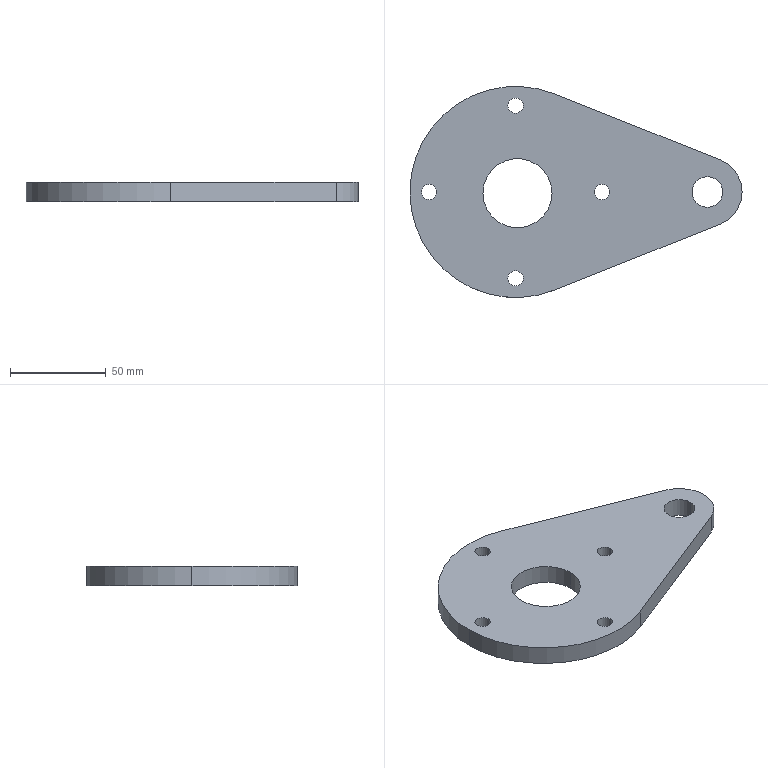Part | STEP file | Anti-vibration sleeve | 1 solid | 19 faces | box 173 x 110 x 10 mm | volume 116462 mm3 | cylinder 15 | plane 4 | commonest cylinder face diameters 8 x8 36 x3 16 x2 110 x2
STEP:
#1=CARTESIAN_POINT('',(48.005,0.6397,10.));
#2=VERTEX_POINT('',#1);
#3=CARTESIAN_POINT('',(40.005,0.6397,10.));
#4=VERTEX_POINT('',#3);
#5=CARTESIAN_POINT('',(44.005,0.6397,10.));
#6=DIRECTION('',(0.,0.,-1.));
#7=DIRECTION('',(-1.,0.,0.));
#8=AXIS2_PLACEMENT_3D('',#5,#6,#7);
#9=CIRCLE('',#8,4.);
#10=EDGE_CURVE('',#2,#4,#9,.T.);
#11=ORIENTED_EDGE('',*,*,#10,.F.);
#12=CARTESIAN_POINT('',(48.005,0.6397,0.));
#13=VERTEX_POINT('',#12);
#14=CARTESIAN_POINT('',(48.005,0.6397,5.));
#15=DIRECTION('',(0.,0.,-1.));
#16=VECTOR('',#15,1000.);
#17=LINE('',#14,#16);
#18=EDGE_CURVE('',#2,#13,#17,.T.);
#19=ORIENTED_EDGE('',*,*,#18,.T.);
#20=CARTESIAN_POINT('',(40.005,0.6397,0.));
#21=VERTEX_POINT('',#20);
#22=CARTESIAN_POINT('',(44.005,0.6397,0.));
#23=DIRECTION('',(0.,0.,1.));
#24=DIRECTION('',(-1.,0.,0.));
#25=AXIS2_PLACEMENT_3D('',#22,#23,#24);
#26=CIRCLE('',#25,4.);
#27=EDGE_CURVE('',#21,#13,#26,.T.);
#28=ORIENTED_EDGE('',*,*,#27,.F.);
#29=CARTESIAN_POINT('',(40.005,0.6397,5.));
#30=DIRECTION('',(0.,0.,-1.));
#31=VECTOR('',#30,1000.);
#32=LINE('',#29,#31);
#33=EDGE_CURVE('',#4,#21,#32,.T.);
#34=ORIENTED_EDGE('',*,*,#33,.F.);
#35=EDGE_LOOP('',(#11,#19,#28,#34));
#36=FACE_OUTER_BOUND('',#35,.T.);
#37=CARTESIAN_POINT('',(44.005,0.6397,5.));
#38=DIRECTION('',(0.,0.,-1.));
#39=DIRECTION('',(-1.,0.,0.));
#40=AXIS2_PLACEMENT_3D('',#37,#38,#39);
#41=CYLINDRICAL_SURFACE('',#40,4.);
#42=ADVANCED_FACE('',(#36),#41,.F.);
#43=CARTESIAN_POINT('',(-41.995,0.6397,10.));
#44=VERTEX_POINT('',#43);
#45=CARTESIAN_POINT('',(-49.995,0.6397,10.));
#46=VERTEX_POINT('',#45);
#47=CARTESIAN_POINT('',(-45.995,0.6397,10.));
#48=DIRECTION('',(0.,0.,-1.));
#49=DIRECTION('',(-1.,0.,0.));
#50=AXIS2_PLACEMENT_3D('',#47,#48,#49);
#51=CIRCLE('',#50,4.);
#52=EDGE_CURVE('',#44,#46,#51,.T.);
#53=ORIENTED_EDGE('',*,*,#52,.F.);
#54=CARTESIAN_POINT('',(-41.995,0.6397,0.));
#55=VERTEX_POINT('',#54);
#56=CARTESIAN_POINT('',(-41.995,0.6397,5.));
#57=DIRECTION('',(0.,0.,-1.));
#58=VECTOR('',#57,1000.);
#59=LINE('',#56,#58);
#60=EDGE_CURVE('',#44,#55,#59,.T.);
#61=ORIENTED_EDGE('',*,*,#60,.T.);
#62=CARTESIAN_POINT('',(-49.995,0.6397,0.));
#63=VERTEX_POINT('',#62);
#64=CARTESIAN_POINT('',(-45.995,0.6397,0.));
#65=DIRECTION('',(0.,0.,1.));
#66=DIRECTION('',(-1.,0.,0.));
#67=AXIS2_PLACEMENT_3D('',#64,#65,#66);
#68=CIRCLE('',#67,4.);
#69=EDGE_CURVE('',#63,#55,#68,.T.);
#70=ORIENTED_EDGE('',*,*,#69,.F.);
#71=CARTESIAN_POINT('',(-49.995,0.6397,5.));
#72=DIRECTION('',(0.,0.,-1.));
#73=VECTOR('',#72,1000.);
#74=LINE('',#71,#73);
#75=EDGE_CURVE('',#46,#63,#74,.T.);
#76=ORIENTED_EDGE('',*,*,#75,.F.);
#77=EDGE_LOOP('',(#53,#61,#70,#76));
#78=FACE_OUTER_BOUND('',#77,.T.);
#79=CARTESIAN_POINT('',(-45.995,0.6397,5.));
#80=DIRECTION('',(0.,0.,-1.));
#81=DIRECTION('',(-1.,0.,0.));
#82=AXIS2_PLACEMENT_3D('',#79,#80,#81);
#83=CYLINDRICAL_SURFACE('',#82,4.);
#84=ADVANCED_FACE('',(#78),#83,.F.);
#85=CARTESIAN_POINT('',(107.005,0.6397,10.));
#86=VERTEX_POINT('',#85);
#87=CARTESIAN_POINT('',(91.005,0.6397,10.));
#88=VERTEX_POINT('',#87);
#89=CARTESIAN_POINT('',(99.005,0.6397,10.));
#90=DIRECTION('',(0.,0.,-1.));
#91=DIRECTION('',(-1.,0.,0.));
#92=AXIS2_PLACEMENT_3D('',#89,#90,#91);
#93=CIRCLE('',#92,8.);
#94=EDGE_CURVE('',#86,#88,#93,.T.);
#95=ORIENTED_EDGE('',*,*,#94,.F.);
#96=CARTESIAN_POINT('',(107.005,0.6397,0.));
#97=VERTEX_POINT('',#96);
#98=CARTESIAN_POINT('',(107.005,0.6397,5.));
#99=DIRECTION('',(0.,0.,-1.));
#100=VECTOR('',#99,1000.);
#101=LINE('',#98,#100);
#102=EDGE_CURVE('',#86,#97,#101,.T.);
#103=ORIENTED_EDGE('',*,*,#102,.T.);
#104=CARTESIAN_POINT('',(91.005,0.6397,0.));
#105=VERTEX_POINT('',#104);
#106=CARTESIAN_POINT('',(99.005,0.6397,0.));
#107=DIRECTION('',(0.,0.,1.));
#108=DIRECTION('',(-1.,0.,0.));
#109=AXIS2_PLACEMENT_3D('',#106,#107,#108);
#110=CIRCLE('',#109,8.);
#111=EDGE_CURVE('',#105,#97,#110,.T.);
#112=ORIENTED_EDGE('',*,*,#111,.F.);
#113=CARTESIAN_POINT('',(91.005,0.6397,5.));
#114=DIRECTION('',(0.,0.,-1.));
#115=VECTOR('',#114,1000.);
#116=LINE('',#113,#115);
#117=EDGE_CURVE('',#88,#105,#116,.T.);
#118=ORIENTED_EDGE('',*,*,#117,.F.);
#119=EDGE_LOOP('',(#95,#103,#112,#118));
#120=FACE_OUTER_BOUND('',#119,.T.);
#121=CARTESIAN_POINT('',(99.005,0.6397,5.));
#122=DIRECTION('',(0.,0.,-1.));
#123=DIRECTION('',(-1.,0.,0.));
#124=AXIS2_PLACEMENT_3D('',#121,#122,#123);
#125=CYLINDRICAL_SURFACE('',#124,8.);
#126=ADVANCED_FACE('',(#120),#125,.F.);
#127=CARTESIAN_POINT('',(-55.995,0.6397,10.));
#128=VERTEX_POINT('',#127);
#129=CARTESIAN_POINT('',(19.355,-50.457,10.));
#130=VERTEX_POINT('',#129);
#131=CARTESIAN_POINT('',(-0.9946,0.6397,10.));
#132=DIRECTION('',(0.,0.,1.));
#133=DIRECTION('',(-1.,0.,0.));
#134=AXIS2_PLACEMENT_3D('',#131,#132,#133);
#135=CIRCLE('',#134,55.);
#136=EDGE_CURVE('',#128,#130,#135,.T.);
#137=ORIENTED_EDGE('',*,*,#136,.F.);
#138=CARTESIAN_POINT('',(-55.995,0.6397,0.));
#139=VERTEX_POINT('',#138);
#140=CARTESIAN_POINT('',(-55.995,0.6397,5.));
#141=DIRECTION('',(0.,0.,-1.));
#142=VECTOR('',#141,1000.);
#143=LINE('',#140,#142);
#144=EDGE_CURVE('',#128,#139,#143,.T.);
#145=ORIENTED_EDGE('',*,*,#144,.T.);
#146=CARTESIAN_POINT('',(19.355,-50.457,0.));
#147=VERTEX_POINT('',#146);
#148=CARTESIAN_POINT('',(-0.9946,0.6397,0.));
#149=DIRECTION('',(0.,0.,1.));
#150=DIRECTION('',(-1.,0.,0.));
#151=AXIS2_PLACEMENT_3D('',#148,#149,#150);
#152=CIRCLE('',#151,55.);
#153=EDGE_CURVE('',#139,#147,#152,.T.);
#154=ORIENTED_EDGE('',*,*,#153,.T.);
#155=CARTESIAN_POINT('',(19.355,-50.457,5.));
#156=DIRECTION('',(0.,0.,1.));
#157=VECTOR('',#156,1000.);
#158=LINE('',#155,#157);
#159=EDGE_CURVE('',#147,#130,#158,.T.);
#160=ORIENTED_EDGE('',*,*,#159,.T.);
#161=EDGE_LOOP('',(#137,#145,#154,#160));
#162=FACE_OUTER_BOUND('',#161,.T.);
#163=CARTESIAN_POINT('',(-0.9946,0.6397,5.));
#164=DIRECTION('',(0.,0.,-1.));
#165=DIRECTION('',(-1.,0.,0.));
#166=AXIS2_PLACEMENT_3D('',#163,#164,#165);
#167=CYLINDRICAL_SURFACE('',#166,55.);
#168=ADVANCED_FACE('',(#162),#167,.T.);
#169=CARTESIAN_POINT('',(3.005,45.64,10.));
#170=VERTEX_POINT('',#169);
#171=CARTESIAN_POINT('',(-4.995,45.64,10.));
#172=VERTEX_POINT('',#171);
#173=CARTESIAN_POINT('',(-0.9946,45.64,10.));
#174=DIRECTION('',(0.,0.,-1.));
#175=DIRECTION('',(-1.,0.,0.));
#176=AXIS2_PLACEMENT_3D('',#173,#174,#175);
#177=CIRCLE('',#176,4.);
#178=EDGE_CURVE('',#170,#172,#177,.T.);
#179=ORIENTED_EDGE('',*,*,#178,.F.);
#180=CARTESIAN_POINT('',(3.005,45.64,0.));
#181=VERTEX_POINT('',#180);
#182=CARTESIAN_POINT('',(3.005,45.64,5.));
#183=DIRECTION('',(0.,0.,-1.));
#184=VECTOR('',#183,1000.);
#185=LINE('',#182,#184);
#186=EDGE_CURVE('',#170,#181,#185,.T.);
#187=ORIENTED_EDGE('',*,*,#186,.T.);
#188=CARTESIAN_POINT('',(-4.995,45.64,0.));
#189=VERTEX_POINT('',#188);
#190=CARTESIAN_POINT('',(-0.9946,45.64,0.));
#191=DIRECTION('',(0.,0.,1.));
#192=DIRECTION('',(-1.,0.,0.));
#193=AXIS2_PLACEMENT_3D('',#190,#191,#192);
#194=CIRCLE('',#193,4.);
#195=EDGE_CURVE('',#189,#181,#194,.T.);
#196=ORIENTED_EDGE('',*,*,#195,.F.);
#197=CARTESIAN_POINT('',(-4.995,45.64,5.));
#198=DIRECTION('',(0.,0.,-1.));
#199=VECTOR('',#198,1000.);
#200=LINE('',#197,#199);
#201=EDGE_CURVE('',#172,#189,#200,.T.);
#202=ORIENTED_EDGE('',*,*,#201,.F.);
#203=EDGE_LOOP('',(#179,#187,#196,#202));
#204=FACE_OUTER_BOUND('',#203,.T.);
#205=CARTESIAN_POINT('',(-0.9946,45.64,5.));
#206=DIRECTION('',(0.,0.,-1.));
#207=DIRECTION('',(-1.,0.,0.));
#208=AXIS2_PLACEMENT_3D('',#205,#206,#207);
#209=CYLINDRICAL_SURFACE('',#208,4.);
#210=ADVANCED_FACE('',(#204),#209,.F.);
#211=CARTESIAN_POINT('',(3.005,-44.36,10.));
#212=VERTEX_POINT('',#211);
#213=CARTESIAN_POINT('',(-4.995,-44.36,10.));
#214=VERTEX_POINT('',#213);
#215=CARTESIAN_POINT('',(-0.9946,-44.36,10.));
#216=DIRECTION('',(0.,0.,-1.));
#217=DIRECTION('',(-1.,0.,0.));
#218=AXIS2_PLACEMENT_3D('',#215,#216,#217);
#219=CIRCLE('',#218,4.);
#220=EDGE_CURVE('',#212,#214,#219,.T.);
#221=ORIENTED_EDGE('',*,*,#220,.F.);
#222=CARTESIAN_POINT('',(3.005,-44.36,0.));
#223=VERTEX_POINT('',#222);
#224=CARTESIAN_POINT('',(3.005,-44.36,5.));
#225=DIRECTION('',(0.,0.,-1.));
#226=VECTOR('',#225,1000.);
#227=LINE('',#224,#226);
#228=EDGE_CURVE('',#212,#223,#227,.T.);
#229=ORIENTED_EDGE('',*,*,#228,.T.);
#230=CARTESIAN_POINT('',(-4.995,-44.36,0.));
#231=VERTEX_POINT('',#230);
#232=CARTESIAN_POINT('',(-0.9946,-44.36,0.));
#233=DIRECTION('',(0.,0.,1.));
#234=DIRECTION('',(-1.,0.,0.));
#235=AXIS2_PLACEMENT_3D('',#232,#233,#234);
#236=CIRCLE('',#235,4.);
#237=EDGE_CURVE('',#231,#223,#236,.T.);
#238=ORIENTED_EDGE('',*,*,#237,.F.);
#239=CARTESIAN_POINT('',(-4.995,-44.36,5.));
#240=DIRECTION('',(0.,0.,-1.));
#241=VECTOR('',#240,1000.);
#242=LINE('',#239,#241);
#243=EDGE_CURVE('',#214,#231,#242,.T.);
#244=ORIENTED_EDGE('',*,*,#243,.F.);
#245=EDGE_LOOP('',(#221,#229,#238,#244));
#246=FACE_OUTER_BOUND('',#245,.T.);
#247=CARTESIAN_POINT('',(-0.9946,-44.36,5.));
#248=DIRECTION('',(0.,0.,-1.));
#249=DIRECTION('',(-1.,0.,0.));
#250=AXIS2_PLACEMENT_3D('',#247,#248,#249);
#251=CYLINDRICAL_SURFACE('',#250,4.);
#252=ADVANCED_FACE('',(#246),#251,.F.);
#253=CARTESIAN_POINT('',(-18.,0.,0.));
#254=VERTEX_POINT('',#253);
#255=CARTESIAN_POINT('',(18.,0.,0.));
#256=VERTEX_POINT('',#255);
#257=CARTESIAN_POINT('',(0.,0.,0.));
#258=DIRECTION('',(0.,0.,1.));
#259=DIRECTION('',(1.,0.,0.));
#260=AXIS2_PLACEMENT_3D('',#257,#258,#259);
#261=CIRCLE('',#260,18.);
#262=EDGE_CURVE('',#254,#256,#261,.T.);
#263=ORIENTED_EDGE('',*,*,#262,.F.);
#264=CARTESIAN_POINT('',(-18.,0.,10.));
#265=VERTEX_POINT('',#264);
#266=CARTESIAN_POINT('',(-18.,0.,0.));
#267=DIRECTION('',(0.,0.,1.));
#268=VECTOR('',#267,1000.);
#269=LINE('',#266,#268);
#270=EDGE_CURVE('',#254,#265,#269,.T.);
#271=ORIENTED_EDGE('',*,*,#270,.T.);
#272=CARTESIAN_POINT('',(18.,0.,10.));
#273=VERTEX_POINT('',#272);
#274=CARTESIAN_POINT('',(0.,0.,10.));
#275=DIRECTION('',(0.,0.,-1.));
#276=DIRECTION('',(1.,0.,0.));
#277=AXIS2_PLACEMENT_3D('',#274,#275,#276);
#278=CIRCLE('',#277,18.);
#279=EDGE_CURVE('',#273,#265,#278,.T.);
#280=ORIENTED_EDGE('',*,*,#279,.F.);
#281=CARTESIAN_POINT('',(18.,0.,0.));
#282=DIRECTION('',(0.,0.,1.));
#283=VECTOR('',#282,1000.);
#284=LINE('',#281,#283);
#285=EDGE_CURVE('',#256,#273,#284,.T.);
#286=ORIENTED_EDGE('',*,*,#285,.F.);
#287=EDGE_LOOP('',(#263,#271,#280,#286));
#288=FACE_OUTER_BOUND('',#287,.T.);
#289=CARTESIAN_POINT('',(0.,0.,0.));
#290=DIRECTION('',(0.,0.,1.));
#291=DIRECTION('',(1.,0.,0.));
#292=AXIS2_PLACEMENT_3D('',#289,#290,#291);
#293=CYLINDRICAL_SURFACE('',#292,18.);
#294=ADVANCED_FACE('',(#288),#293,.F.);
#295=CARTESIAN_POINT('',(44.005,0.6397,10.));
#296=DIRECTION('',(0.,0.,-1.));
#297=DIRECTION('',(-1.,0.,0.));
#298=AXIS2_PLACEMENT_3D('',#295,#296,#297);
#299=CIRCLE('',#298,4.);
#300=EDGE_CURVE('',#4,#2,#299,.T.);
#301=ORIENTED_EDGE('',*,*,#300,.T.);
#302=ORIENTED_EDGE('',*,*,#10,.T.);
#303=EDGE_LOOP('',(#301,#302));
#304=FACE_BOUND('',#303,.T.);
#305=CARTESIAN_POINT('',(-45.995,0.6397,10.));
#306=DIRECTION('',(0.,0.,-1.));
#307=DIRECTION('',(-1.,0.,0.));
#308=AXIS2_PLACEMENT_3D('',#305,#306,#307);
#309=CIRCLE('',#308,4.);
#310=EDGE_CURVE('',#46,#44,#309,.T.);
#311=ORIENTED_EDGE('',*,*,#310,.T.);
#312=ORIENTED_EDGE('',*,*,#52,.T.);
#313=EDGE_LOOP('',(#311,#312));
#314=FACE_BOUND('',#313,.T.);
#315=CARTESIAN_POINT('',(99.005,0.6397,10.));
#316=DIRECTION('',(0.,0.,-1.));
#317=DIRECTION('',(-1.,0.,0.));
#318=AXIS2_PLACEMENT_3D('',#315,#316,#317);
#319=CIRCLE('',#318,8.);
#320=EDGE_CURVE('',#88,#86,#319,.T.);
#321=ORIENTED_EDGE('',*,*,#320,.T.);
#322=ORIENTED_EDGE('',*,*,#94,.T.);
#323=EDGE_LOOP('',(#321,#322));
#324=FACE_BOUND('',#323,.T.);
#325=CARTESIAN_POINT('',(19.355,51.736,10.));
#326=VERTEX_POINT('',#325);
#327=CARTESIAN_POINT('',(-0.9946,0.6397,10.));
#328=DIRECTION('',(0.,0.,1.));
#329=DIRECTION('',(-1.,0.,0.));
#330=AXIS2_PLACEMENT_3D('',#327,#328,#329);
#331=CIRCLE('',#330,55.);
#332=EDGE_CURVE('',#326,#128,#331,.T.);
#333=ORIENTED_EDGE('',*,*,#332,.T.);
#334=ORIENTED_EDGE('',*,*,#136,.T.);
#335=CARTESIAN_POINT('',(105.665,-16.083,10.));
#336=VERTEX_POINT('',#335);
#337=CARTESIAN_POINT('',(19.355,-50.457,10.));
#338=DIRECTION('',(0.929,0.37,0.));
#339=VECTOR('',#338,1000.);
#340=LINE('',#337,#339);
#341=EDGE_CURVE('',#130,#336,#340,.T.);
#342=ORIENTED_EDGE('',*,*,#341,.T.);
#343=CARTESIAN_POINT('',(105.665,17.362,10.));
#344=VERTEX_POINT('',#343);
#345=CARTESIAN_POINT('',(99.005,0.6397,10.));
#346=DIRECTION('',(0.,0.,1.));
#347=DIRECTION('',(-1.,0.,0.));
#348=AXIS2_PLACEMENT_3D('',#345,#346,#347);
#349=CIRCLE('',#348,18.);
#350=EDGE_CURVE('',#336,#344,#349,.T.);
#351=ORIENTED_EDGE('',*,*,#350,.T.);
#352=CARTESIAN_POINT('',(105.665,17.362,10.));
#353=DIRECTION('',(-0.929,0.37,0.));
#354=VECTOR('',#353,1000.);
#355=LINE('',#352,#354);
#356=EDGE_CURVE('',#344,#326,#355,.T.);
#357=ORIENTED_EDGE('',*,*,#356,.T.);
#358=EDGE_LOOP('',(#333,#334,#342,#351,#357));
#359=FACE_OUTER_BOUND('',#358,.T.);
#360=CARTESIAN_POINT('',(-0.9946,45.64,10.));
#361=DIRECTION('',(0.,0.,-1.));
#362=DIRECTION('',(-1.,0.,0.));
#363=AXIS2_PLACEMENT_3D('',#360,#361,#362);
#364=CIRCLE('',#363,4.);
#365=EDGE_CURVE('',#172,#170,#364,.T.);
#366=ORIENTED_EDGE('',*,*,#365,.T.);
#367=ORIENTED_EDGE('',*,*,#178,.T.);
#368=EDGE_LOOP('',(#366,#367));
#369=FACE_BOUND('',#368,.T.);
#370=CARTESIAN_POINT('',(-0.9946,-44.36,10.));
#371=DIRECTION('',(0.,0.,-1.));
#372=DIRECTION('',(-1.,0.,0.));
#373=AXIS2_PLACEMENT_3D('',#370,#371,#372);
#374=CIRCLE('',#373,4.);
#375=EDGE_CURVE('',#214,#212,#374,.T.);
#376=ORIENTED_EDGE('',*,*,#375,.T.);
#377=ORIENTED_EDGE('',*,*,#220,.T.);
#378=EDGE_LOOP('',(#376,#377));
#379=FACE_BOUND('',#378,.T.);
#380=ORIENTED_EDGE('',*,*,#279,.T.);
#381=CARTESIAN_POINT('',(0.,0.,10.));
#382=DIRECTION('',(0.,0.,-1.));
#383=DIRECTION('',(1.,0.,0.));
#384=AXIS2_PLACEMENT_3D('',#381,#382,#383);
#385=CIRCLE('',#384,18.);
#386=EDGE_CURVE('',#265,#273,#385,.T.);
#387=ORIENTED_EDGE('',*,*,#386,.T.);
#388=EDGE_LOOP('',(#380,#387));
#389=FACE_BOUND('',#388,.T.);
#390=CARTESIAN_POINT('',(99.005,0.6397,10.));
#391=DIRECTION('',(0.,0.,1.));
#392=DIRECTION('',(1.,0.,0.));
#393=AXIS2_PLACEMENT_3D('',#390,#391,#392);
#394=PLANE('',#393);
#395=ADVANCED_FACE('',(#304,#314,#324,#359,#369,#379,#389),#394,.T.);
#396=ORIENTED_EDGE('',*,*,#18,.F.);
#397=ORIENTED_EDGE('',*,*,#300,.F.);
#398=ORIENTED_EDGE('',*,*,#33,.T.);
#399=CARTESIAN_POINT('',(44.005,0.6397,0.));
#400=DIRECTION('',(0.,0.,1.));
#401=DIRECTION('',(-1.,0.,0.));
#402=AXIS2_PLACEMENT_3D('',#399,#400,#401);
#403=CIRCLE('',#402,4.);
#404=EDGE_CURVE('',#13,#21,#403,.T.);
#405=ORIENTED_EDGE('',*,*,#404,.F.);
#406=EDGE_LOOP('',(#396,#397,#398,#405));
#407=FACE_OUTER_BOUND('',#406,.T.);
#408=CARTESIAN_POINT('',(44.005,0.6397,5.));
#409=DIRECTION('',(0.,0.,-1.));
#410=DIRECTION('',(-1.,0.,0.));
#411=AXIS2_PLACEMENT_3D('',#408,#409,#410);
#412=CYLINDRICAL_SURFACE('',#411,4.);
#413=ADVANCED_FACE('',(#407),#412,.F.);
#414=ORIENTED_EDGE('',*,*,#60,.F.);
#415=ORIENTED_EDGE('',*,*,#310,.F.);
#416=ORIENTED_EDGE('',*,*,#75,.T.);
#417=CARTESIAN_POINT('',(-45.995,0.6397,0.));
#418=DIRECTION('',(0.,0.,1.));
#419=DIRECTION('',(-1.,0.,0.));
#420=AXIS2_PLACEMENT_3D('',#417,#418,#419);
#421=CIRCLE('',#420,4.);
#422=EDGE_CURVE('',#55,#63,#421,.T.);
#423=ORIENTED_EDGE('',*,*,#422,.F.);
#424=EDGE_LOOP('',(#414,#415,#416,#423));
#425=FACE_OUTER_BOUND('',#424,.T.);
#426=CARTESIAN_POINT('',(-45.995,0.6397,5.));
#427=DIRECTION('',(0.,0.,-1.));
#428=DIRECTION('',(-1.,0.,0.));
#429=AXIS2_PLACEMENT_3D('',#426,#427,#428);
#430=CYLINDRICAL_SURFACE('',#429,4.);
#431=ADVANCED_FACE('',(#425),#430,.F.);
#432=ORIENTED_EDGE('',*,*,#102,.F.);
#433=ORIENTED_EDGE('',*,*,#320,.F.);
#434=ORIENTED_EDGE('',*,*,#117,.T.);
#435=CARTESIAN_POINT('',(99.005,0.6397,0.));
#436=DIRECTION('',(0.,0.,1.));
#437=DIRECTION('',(-1.,0.,0.));
#438=AXIS2_PLACEMENT_3D('',#435,#436,#437);
#439=CIRCLE('',#438,8.);
#440=EDGE_CURVE('',#97,#105,#439,.T.);
#441=ORIENTED_EDGE('',*,*,#440,.F.);
#442=EDGE_LOOP('',(#432,#433,#434,#441));
#443=FACE_OUTER_BOUND('',#442,.T.);
#444=CARTESIAN_POINT('',(99.005,0.6397,5.));
#445=DIRECTION('',(0.,0.,-1.));
#446=DIRECTION('',(-1.,0.,0.));
#447=AXIS2_PLACEMENT_3D('',#444,#445,#446);
#448=CYLINDRICAL_SURFACE('',#447,8.);
#449=ADVANCED_FACE('',(#443),#448,.F.);
#450=CARTESIAN_POINT('',(105.665,-16.083,0.));
#451=VERTEX_POINT('',#450);
#452=CARTESIAN_POINT('',(105.665,-16.083,5.));
#453=DIRECTION('',(0.,0.,-1.));
#454=VECTOR('',#453,1000.);
#455=LINE('',#452,#454);
#456=EDGE_CURVE('',#336,#451,#455,.T.);
#457=ORIENTED_EDGE('',*,*,#456,.F.);
#458=ORIENTED_EDGE('',*,*,#341,.F.);
#459=ORIENTED_EDGE('',*,*,#159,.F.);
#460=CARTESIAN_POINT('',(19.355,-50.457,0.));
#461=DIRECTION('',(-0.929,-0.37,0.));
#462=VECTOR('',#461,1000.);
#463=LINE('',#460,#462);
#464=EDGE_CURVE('',#451,#147,#463,.T.);
#465=ORIENTED_EDGE('',*,*,#464,.F.);
#466=EDGE_LOOP('',(#457,#458,#459,#465));
#467=FACE_OUTER_BOUND('',#466,.T.);
#468=CARTESIAN_POINT('',(19.355,-50.457,5.));
#469=DIRECTION('',(-0.37,0.929,0.));
#470=DIRECTION('',(-0.929,-0.37,0.));
#471=AXIS2_PLACEMENT_3D('',#468,#469,#470);
#472=PLANE('',#471);
#473=ADVANCED_FACE('',(#467),#472,.F.);
#474=ORIENTED_EDGE('',*,*,#144,.F.);
#475=ORIENTED_EDGE('',*,*,#332,.F.);
#476=CARTESIAN_POINT('',(19.355,51.736,0.));
#477=VERTEX_POINT('',#476);
#478=CARTESIAN_POINT('',(19.355,51.736,5.));
#479=DIRECTION('',(0.,0.,-1.));
#480=VECTOR('',#479,1000.);
#481=LINE('',#478,#480);
#482=EDGE_CURVE('',#326,#477,#481,.T.);
#483=ORIENTED_EDGE('',*,*,#482,.T.);
#484=CARTESIAN_POINT('',(-0.9946,0.6397,0.));
#485=DIRECTION('',(0.,0.,1.));
#486=DIRECTION('',(-1.,0.,0.));
#487=AXIS2_PLACEMENT_3D('',#484,#485,#486);
#488=CIRCLE('',#487,55.);
#489=EDGE_CURVE('',#477,#139,#488,.T.);
#490=ORIENTED_EDGE('',*,*,#489,.T.);
#491=EDGE_LOOP('',(#474,#475,#483,#490));
#492=FACE_OUTER_BOUND('',#491,.T.);
#493=CARTESIAN_POINT('',(-0.9946,0.6397,5.));
#494=DIRECTION('',(0.,0.,-1.));
#495=DIRECTION('',(-1.,0.,0.));
#496=AXIS2_PLACEMENT_3D('',#493,#494,#495);
#497=CYLINDRICAL_SURFACE('',#496,55.);
#498=ADVANCED_FACE('',(#492),#497,.T.);
#499=ORIENTED_EDGE('',*,*,#482,.F.);
#500=ORIENTED_EDGE('',*,*,#356,.F.);
#501=CARTESIAN_POINT('',(105.665,17.362,0.));
#502=VERTEX_POINT('',#501);
#503=CARTESIAN_POINT('',(105.665,17.362,5.));
#504=DIRECTION('',(0.,0.,1.));
#505=VECTOR('',#504,1000.);
#506=LINE('',#503,#505);
#507=EDGE_CURVE('',#502,#344,#506,.T.);
#508=ORIENTED_EDGE('',*,*,#507,.F.);
#509=CARTESIAN_POINT('',(19.355,51.736,0.));
#510=DIRECTION('',(0.929,-0.37,0.));
#511=VECTOR('',#510,1000.);
#512=LINE('',#509,#511);
#513=EDGE_CURVE('',#477,#502,#512,.T.);
#514=ORIENTED_EDGE('',*,*,#513,.F.);
#515=EDGE_LOOP('',(#499,#500,#508,#514));
#516=FACE_OUTER_BOUND('',#515,.T.);
#517=CARTESIAN_POINT('',(19.355,51.736,5.));
#518=DIRECTION('',(-0.37,-0.929,0.));
#519=DIRECTION('',(0.929,-0.37,0.));
#520=AXIS2_PLACEMENT_3D('',#517,#518,#519);
#521=PLANE('',#520);
#522=ADVANCED_FACE('',(#516),#521,.F.);
#523=ORIENTED_EDGE('',*,*,#350,.F.);
#524=ORIENTED_EDGE('',*,*,#456,.T.);
#525=CARTESIAN_POINT('',(99.005,0.6397,0.));
#526=DIRECTION('',(0.,0.,1.));
#527=DIRECTION('',(-1.,0.,0.));
#528=AXIS2_PLACEMENT_3D('',#525,#526,#527);
#529=CIRCLE('',#528,18.);
#530=EDGE_CURVE('',#451,#502,#529,.T.);
#531=ORIENTED_EDGE('',*,*,#530,.T.);
#532=ORIENTED_EDGE('',*,*,#507,.T.);
#533=EDGE_LOOP('',(#523,#524,#531,#532));
#534=FACE_OUTER_BOUND('',#533,.T.);
#535=CARTESIAN_POINT('',(99.005,0.6397,5.));
#536=DIRECTION('',(0.,0.,-1.));
#537=DIRECTION('',(-1.,0.,0.));
#538=AXIS2_PLACEMENT_3D('',#535,#536,#537);
#539=CYLINDRICAL_SURFACE('',#538,18.);
#540=ADVANCED_FACE('',(#534),#539,.T.);
#541=ORIENTED_EDGE('',*,*,#186,.F.);
#542=ORIENTED_EDGE('',*,*,#365,.F.);
#543=ORIENTED_EDGE('',*,*,#201,.T.);
#544=CARTESIAN_POINT('',(-0.9946,45.64,0.));
#545=DIRECTION('',(0.,0.,1.));
#546=DIRECTION('',(-1.,0.,0.));
#547=AXIS2_PLACEMENT_3D('',#544,#545,#546);
#548=CIRCLE('',#547,4.);
#549=EDGE_CURVE('',#181,#189,#548,.T.);
#550=ORIENTED_EDGE('',*,*,#549,.F.);
#551=EDGE_LOOP('',(#541,#542,#543,#550));
#552=FACE_OUTER_BOUND('',#551,.T.);
#553=CARTESIAN_POINT('',(-0.9946,45.64,5.));
#554=DIRECTION('',(0.,0.,-1.));
#555=DIRECTION('',(-1.,0.,0.));
#556=AXIS2_PLACEMENT_3D('',#553,#554,#555);
#557=CYLINDRICAL_SURFACE('',#556,4.);
#558=ADVANCED_FACE('',(#552),#557,.F.);
#559=ORIENTED_EDGE('',*,*,#228,.F.);
#560=ORIENTED_EDGE('',*,*,#375,.F.);
#561=ORIENTED_EDGE('',*,*,#243,.T.);
#562=CARTESIAN_POINT('',(-0.9946,-44.36,0.));
#563=DIRECTION('',(0.,0.,1.));
#564=DIRECTION('',(-1.,0.,0.));
#565=AXIS2_PLACEMENT_3D('',#562,#563,#564);
#566=CIRCLE('',#565,4.);
#567=EDGE_CURVE('',#223,#231,#566,.T.);
#568=ORIENTED_EDGE('',*,*,#567,.F.);
#569=EDGE_LOOP('',(#559,#560,#561,#568));
#570=FACE_OUTER_BOUND('',#569,.T.);
#571=CARTESIAN_POINT('',(-0.9946,-44.36,5.));
#572=DIRECTION('',(0.,0.,-1.));
#573=DIRECTION('',(-1.,0.,0.));
#574=AXIS2_PLACEMENT_3D('',#571,#572,#573);
#575=CYLINDRICAL_SURFACE('',#574,4.);
#576=ADVANCED_FACE('',(#570),#575,.F.);
#577=ORIENTED_EDGE('',*,*,#270,.F.);
#578=CARTESIAN_POINT('',(0.,0.,0.));
#579=DIRECTION('',(0.,0.,1.));
#580=DIRECTION('',(1.,0.,0.));
#581=AXIS2_PLACEMENT_3D('',#578,#579,#580);
#582=CIRCLE('',#581,18.);
#583=EDGE_CURVE('',#256,#254,#582,.T.);
#584=ORIENTED_EDGE('',*,*,#583,.F.);
#585=ORIENTED_EDGE('',*,*,#285,.T.);
#586=ORIENTED_EDGE('',*,*,#386,.F.);
#587=EDGE_LOOP('',(#577,#584,#585,#586));
#588=FACE_OUTER_BOUND('',#587,.T.);
#589=CARTESIAN_POINT('',(0.,0.,0.));
#590=DIRECTION('',(0.,0.,1.));
#591=DIRECTION('',(1.,0.,0.));
#592=AXIS2_PLACEMENT_3D('',#589,#590,#591);
#593=CYLINDRICAL_SURFACE('',#592,18.);
#594=ADVANCED_FACE('',(#588),#593,.F.);
#595=ORIENTED_EDGE('',*,*,#27,.T.);
#596=ORIENTED_EDGE('',*,*,#404,.T.);
#597=EDGE_LOOP('',(#595,#596));
#598=FACE_BOUND('',#597,.T.);
#599=ORIENTED_EDGE('',*,*,#69,.T.);
#600=ORIENTED_EDGE('',*,*,#422,.T.);
#601=EDGE_LOOP('',(#599,#600));
#602=FACE_BOUND('',#601,.T.);
#603=ORIENTED_EDGE('',*,*,#111,.T.);
#604=ORIENTED_EDGE('',*,*,#440,.T.);
#605=EDGE_LOOP('',(#603,#604));
#606=FACE_BOUND('',#605,.T.);
#607=ORIENTED_EDGE('',*,*,#464,.T.);
#608=ORIENTED_EDGE('',*,*,#153,.F.);
#609=ORIENTED_EDGE('',*,*,#489,.F.);
#610=ORIENTED_EDGE('',*,*,#513,.T.);
#611=ORIENTED_EDGE('',*,*,#530,.F.);
#612=EDGE_LOOP('',(#607,#608,#609,#610,#611));
#613=FACE_OUTER_BOUND('',#612,.T.);
#614=ORIENTED_EDGE('',*,*,#195,.T.);
#615=ORIENTED_EDGE('',*,*,#549,.T.);
#616=EDGE_LOOP('',(#614,#615));
#617=FACE_BOUND('',#616,.T.);
#618=ORIENTED_EDGE('',*,*,#237,.T.);
#619=ORIENTED_EDGE('',*,*,#567,.T.);
#620=EDGE_LOOP('',(#618,#619));
#621=FACE_BOUND('',#620,.T.);
#622=ORIENTED_EDGE('',*,*,#583,.T.);
#623=ORIENTED_EDGE('',*,*,#262,.T.);
#624=EDGE_LOOP('',(#622,#623));
#625=FACE_BOUND('',#624,.T.);
#626=CARTESIAN_POINT('',(99.005,0.6397,0.));
#627=DIRECTION('',(0.,0.,1.));
#628=DIRECTION('',(1.,0.,0.));
#629=AXIS2_PLACEMENT_3D('',#626,#627,#628);
#630=PLANE('',#629);
#631=ADVANCED_FACE('',(#598,#602,#606,#613,#617,#621,#625),#630,.F.);
#632=CLOSED_SHELL('',(#42,#84,#126,#168,#210,#252,#294,#395,#413,#431,#449,#473,#498,#522,#540,#558,#576,#594,#631));
#633=MANIFOLD_SOLID_BREP('',#632);
#634=CARTESIAN_POINT('',(0.,0.,0.));
#635=DIRECTION('',(0.,0.,1.));
#636=DIRECTION('',(1.,0.,0.));
#637=AXIS2_PLACEMENT_3D('',#634,#635,#636);
#638=(LENGTH_UNIT()NAMED_UNIT(*)SI_UNIT(.MILLI.,.METRE.));
#639=UNCERTAINTY_MEASURE_WITH_UNIT(LENGTH_MEASURE(0.00001),#638,'','');
#640=(NAMED_UNIT(*)PLANE_ANGLE_UNIT()SI_UNIT($,.RADIAN.));
#641=(NAMED_UNIT(*)SI_UNIT($,.STERADIAN.)SOLID_ANGLE_UNIT());
#642=(GEOMETRIC_REPRESENTATION_CONTEXT(3)GLOBAL_UNCERTAINTY_ASSIGNED_CONTEXT((#639))GLOBAL_UNIT_ASSIGNED_CONTEXT((#638,#640,#641))REPRESENTATION_CONTEXT('',''));
#643=ADVANCED_BREP_SHAPE_REPRESENTATION('',(#633,#637),#642);